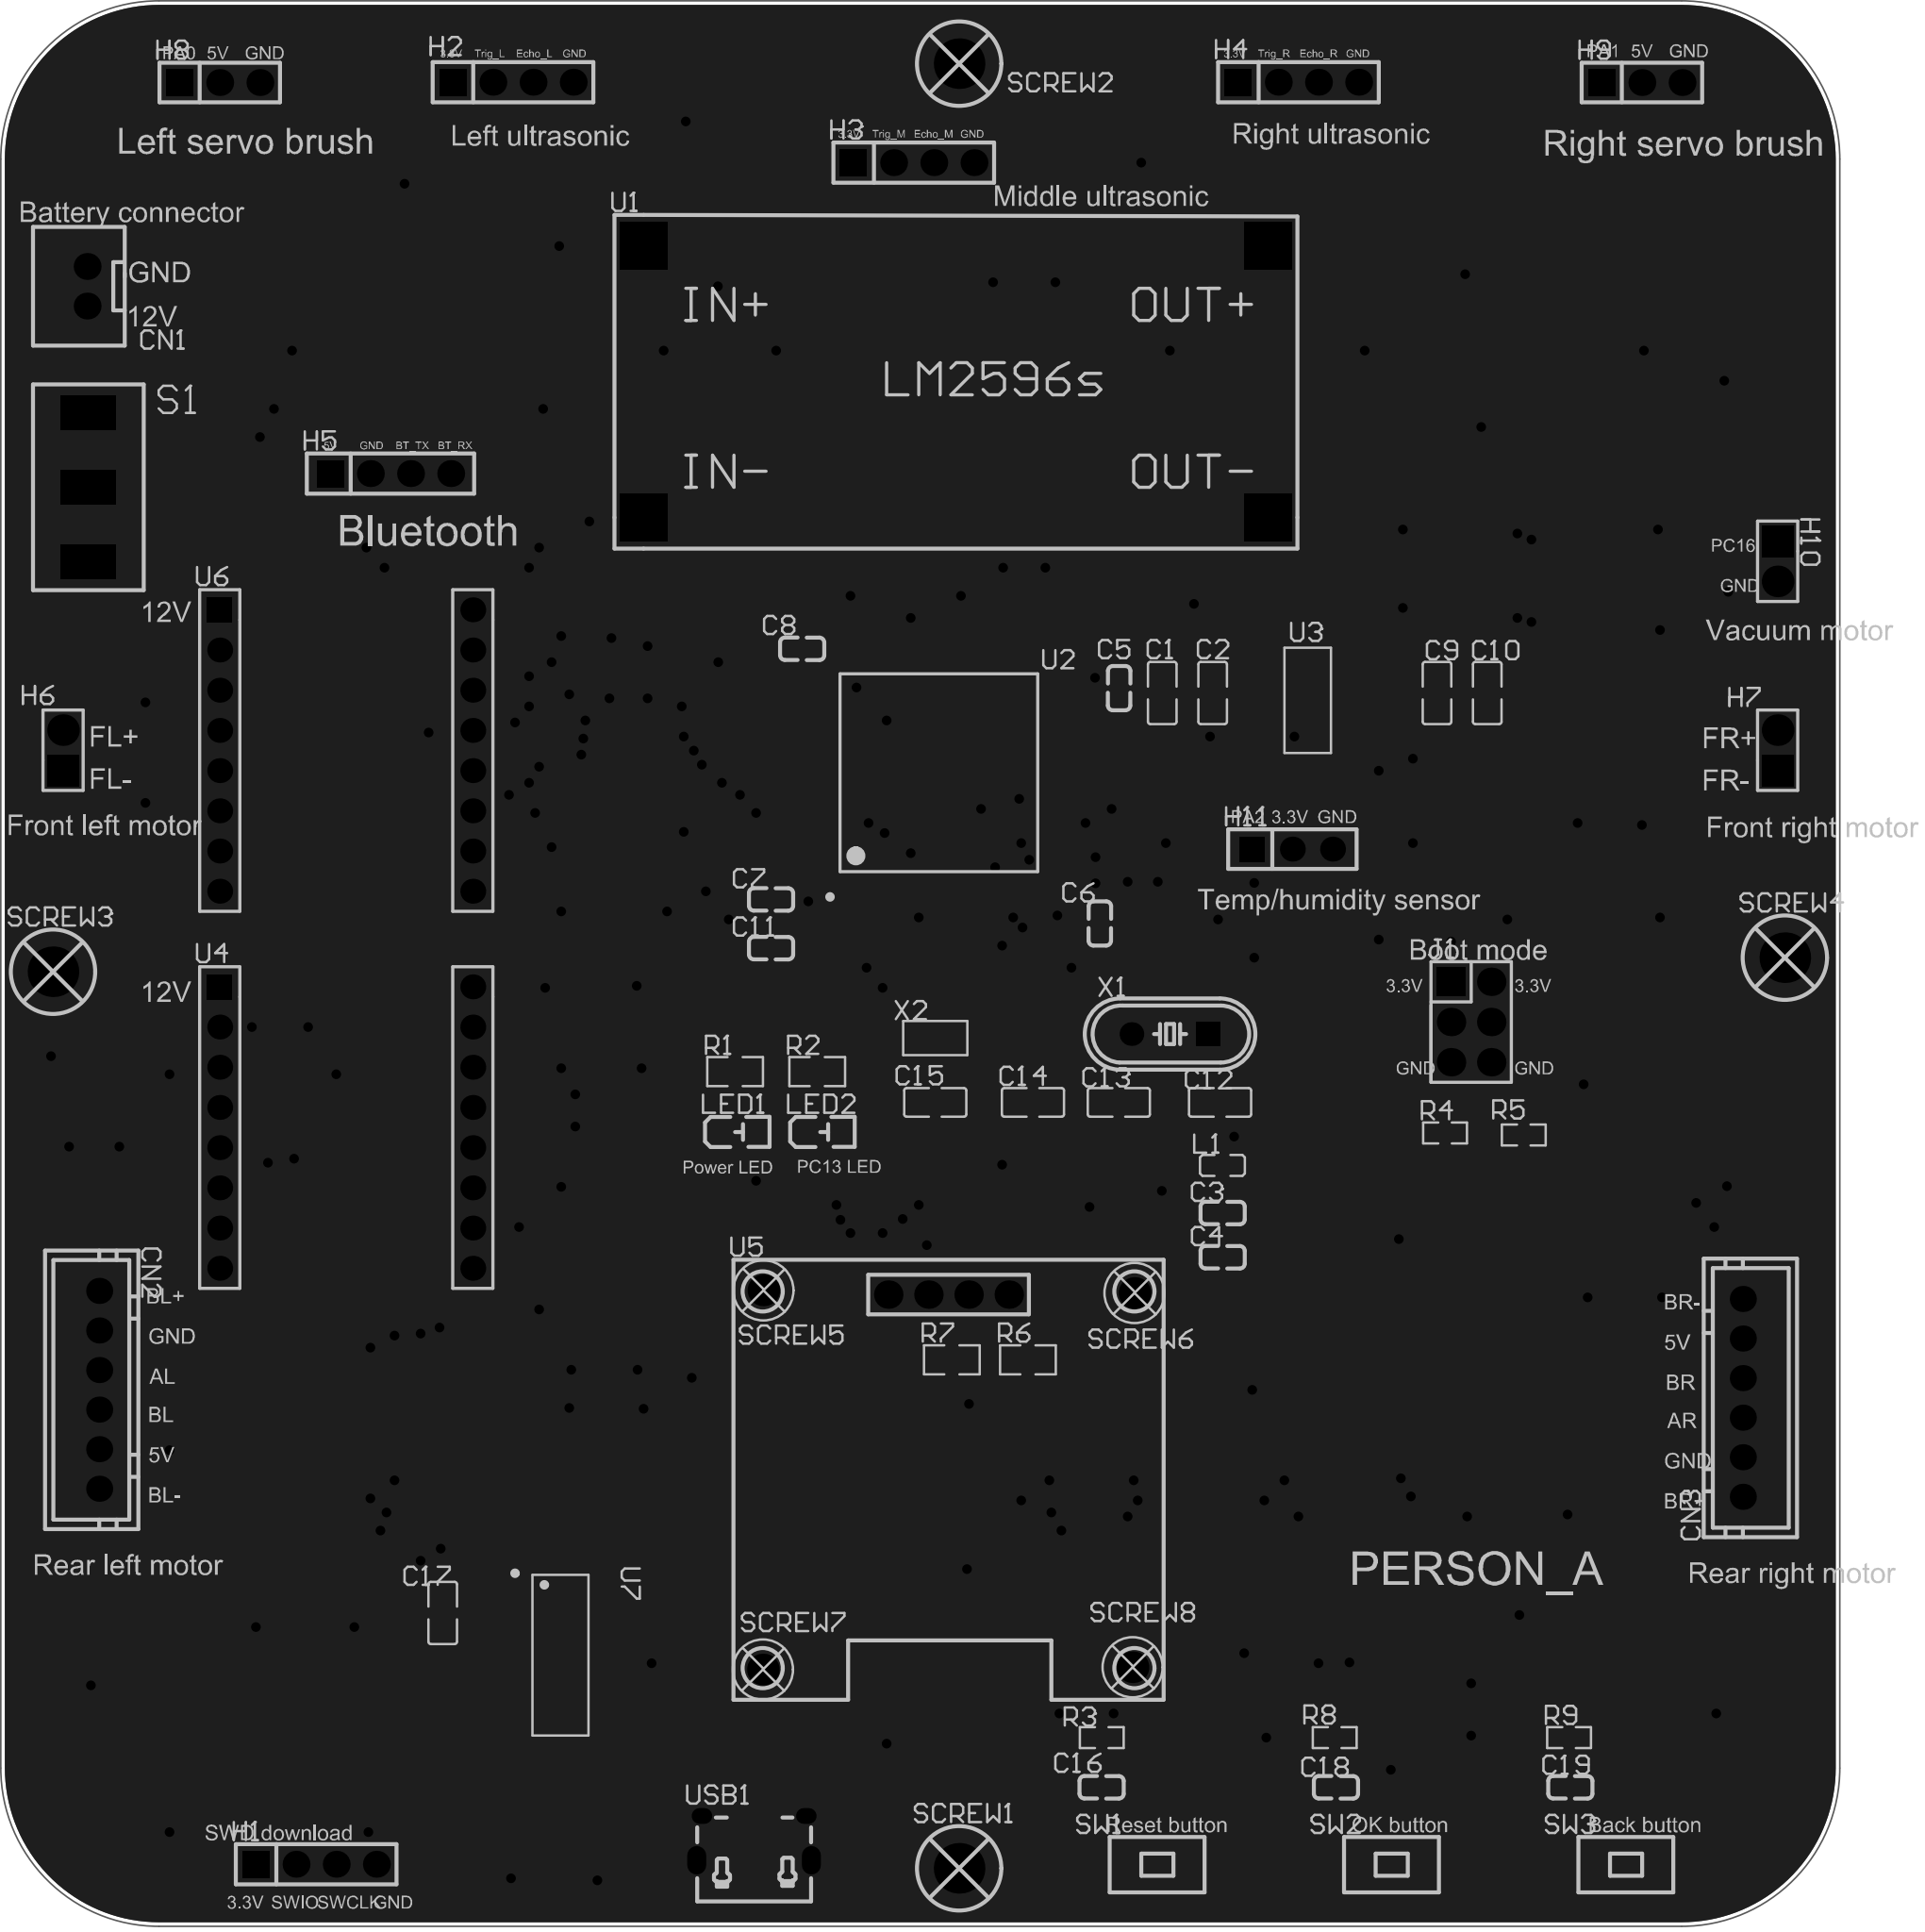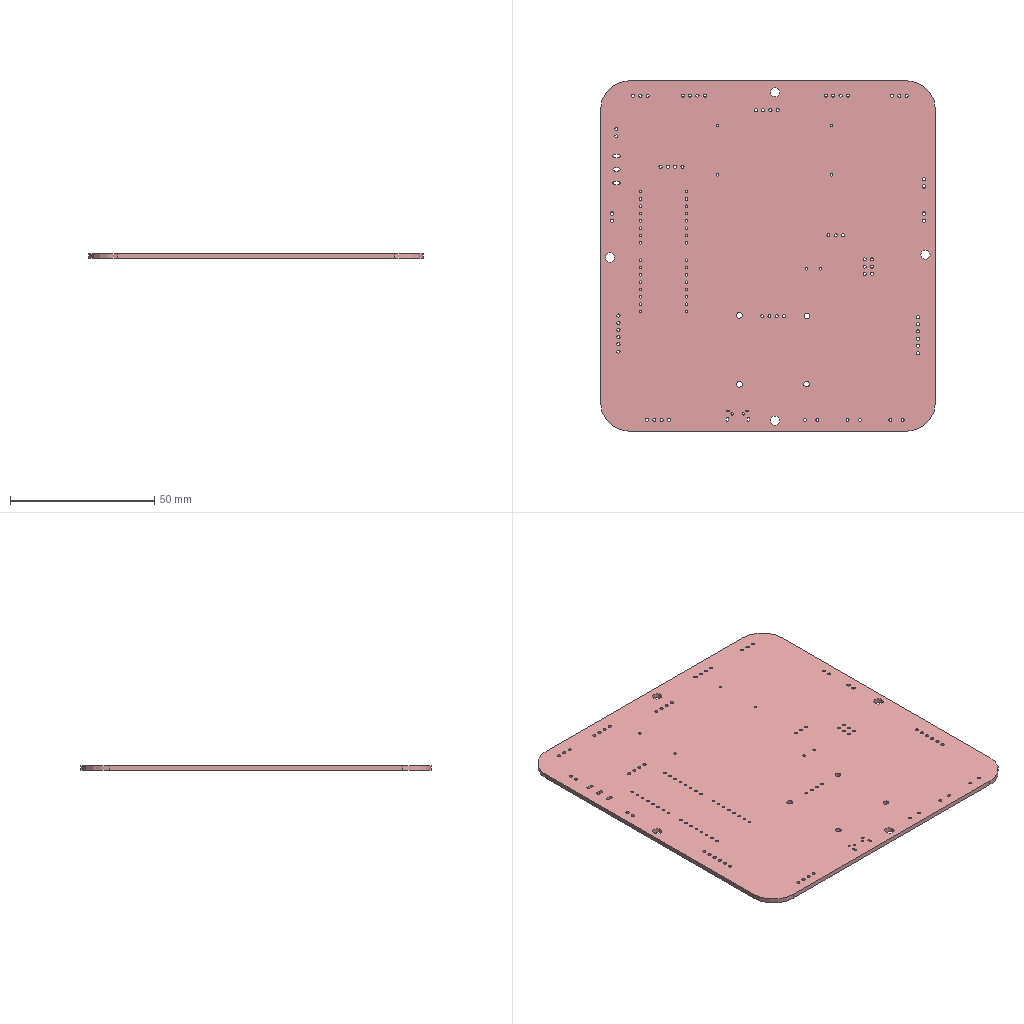Circuit board layout | Altium Designer | box 116.3 x 121.7 x 1.6 mm
Layer stack:
# Altium Designer layer stack of  (unit mm; dielectric type: 0 none, 1 core, 2 prepreg, 3 surface material)
index,name,kind,layer,copper_thickness_mm,dielectric_type,dielectric_thickness_mm,dielectric_material,dielectric_constant
0,Top Paste Mask Layer,other,,,,,,
1,Top Silkscreen Layer,other,,,,,,
2,Top Solder Mask Layer,dielectric,,,3,0.01,,3.3
3,Top Layer,copper,Top Layer,0.035,,,,
4,Dielectric1,dielectric,,,3,1.51,FR4,4.5
5,Bottom Layer,copper,Bottom Layer,0.035,,,,
6,Bottom Solder Mask Layer,dielectric,,,3,0.01,,3.3
7,Bottom Silkscreen Layer,other,,,,,,
8,Bottom Paste Mask Layer,other,,,,,,
# drill layer pairs: low layer,high layer
drill_pair,Top Layer,Bottom Layer
Part placement:
Designator,Comment,Layer,Footprint,Center-X(mm),Center-Y(mm),Rotation
C3,100nF,TopLayer,C0603,160.302,131.826,180
C4,10uF,TopLayer,C0603,160.302,129.032,180
C11,100nF,TopLayer,C0603,131.75,148.558,180
C5,100nF,TopLayer,C0603,153.762,164.975,270
C6,100nF,TopLayer,C0603,152.542,150.108,270
C7,100nF,TopLayer,C0603,131.75,151.638,180
C8,100nF,TopLayer,C0603,133.717,167.471,180
C16,1uF,TopLayer,C0603,152.649,95.543,180
CN1,XH2.54*2P_THT,TopLayer,CONN-TH_2P-P2.50-XH2.54-2P,88.519,190.373,270
CN2,Rear left motor,TopLayer,CONN-TH_XH2.54-6P,89.281,120.651,270
CN3,Rear right motor,TopLayer,CONN-TH_XH2.54-6P,193.199,120.142,90
SCREW1,,TopLayer,M3螺丝,143.65,90.421,0
H1,SWD,TopLayer,HDR-TH_4P-P2.54-V-M,102.997,90.678,0
H5,2.54-1*4P female,TopLayer,HDR-TH_4P-P2.54-V-F,107.696,178.539,0
H6,Front left motor,TopLayer,HDR-TH_2P-P2.54-V-M,86.995,161.061,90
H7,Front right motor,TopLayer,HDR-TH_2P-P2.54-V-M,195.398,161.061,90
H2,Ultrasonic left,TopLayer,HDR-TH_4P-P2.54-V-M,115.442,203.265,0
H3,Ultrasonic middle,TopLayer,HDR-TH_4P-P2.54-V-M,140.78,198.185,0
H4,Ultrasonic right,TopLayer,HDR-TH_4P-P2.54-V-M,165.101,203.265,0
H8,PZ254V-11-03P,TopLayer,HDR-TH_3P-P2.54-V-M,96.901,203.245,0
H9,PZ254V-11-03P,TopLayer,HDR-TH_3P-P2.54-V-M,186.817,203.245,0
H10,PZ254V-11-02P,TopLayer,HDR-TH_2P-P2.54-V-M,195.398,172.998,270
H11,PM254V-11-03-H85,TopLayer,HDR-TH_3P-P2.54-V-F,164.719,154.813,0
J1,2.54-2*3P male pin,TopLayer,HDR-TH_6P-P2.54-V-M-R2-C3-S2.54-1,176.022,143.891,270
L1,10uH,TopLayer,L0603,160.302,134.82,0
LED2,NCD0805R1,TopLayer,LED0805-RD_RED,135.066,136.942,0
LED1,NCD0805R1,TopLayer,LED0805-RD_RED,129.683,136.942,0
R3,10kΩ,TopLayer,R0603,152.666,98.679,0
R5,10kΩ,TopLayer,R0603,179.348,136.752,0
R4,10kΩ,TopLayer,R0603,174.371,136.879,0
R6,4.7kΩ,TopLayer,R0805,147.998,122.546,180
R7,4.7kΩ,TopLayer,R0805,143.188,122.546,180
S1,ss12d10 switch,TopLayer,SS12D10,88.594,177.673,90
SCREW2,,TopLayer,M3螺丝,143.65,204.438,0
U2,STM32F103VET6,TopLayer,LQFP-100_L14.0-W14.0-P0.50-LS16.0-BL,142.367,159.639,0
U3,AMS1117-3.3,TopLayer,SOT-223-3_L6.5-W3.4-P2.30-LS7.0-BR,165.787,164.211,0
U1,LM2596S buck module,TopLayer,LM2596S,143.446,184.34,0
U5,HS96L03W2C03,TopLayer,OLED-TH_L27.8-W27.2-P2.54_C9900033791,142.98,126.669,0
U4,TB6612 module,TopLayer,TB6612-2X8,104.901,137.222,0
U6,TB6612 module,TopLayer,TB6612-2X8,104.901,161.042,0
X1,-,TopLayer,HC-49US_L11.5-W4.5-P4.88,156.985,143.129,180
X2,32.768kHz,TopLayer,OSC-SMD_L3.2-W1.5,142.14,142.875,180
SCREW3,,TopLayer,M3螺丝,86.36,147.066,0
SCREW4,,TopLayer,M3螺丝,195.855,147.955,0
SCREW5,,TopLayer,M2螺丝,131.275,126.935,0
SCREW6,,TopLayer,M2螺丝,154.736,126.769,0
SCREW7,,TopLayer,M2螺丝,131.244,102.981,0
SCREW8,,TopLayer,M2螺丝,154.617,103.124,0
C9,10uF,TopLayer,C0805,173.863,164.675,90
C10,100nF,TopLayer,C0805,177.038,164.675,90
C1,10uF,TopLayer,C0805,156.491,164.675,90
C2,100nF,TopLayer,C0805,159.677,164.675,90
C17,100pF,TopLayer,C0805,110.998,106.553,270
C12,20pF,TopLayer,C0805,160.147,138.811,0
C13,20pF,TopLayer,C0805,153.745,138.811,0
C14,20pF,TopLayer,C0805,148.315,138.811,0
C15,20pF,TopLayer,C0805,142.14,138.811,180
SW1,1TS002C-2300-4300-CT,TopLayer,SW-SMD_L6.0-W3.5-LS8.0-EH,156.166,90.65,0
C18,1uF,TopLayer,C0603,167.466,95.543,180
C19,1uF,TopLayer,C0603,182.283,95.543,180
R8,10kΩ,TopLayer,R0603,167.395,98.679,0
R9,10kΩ,TopLayer,R0603,182.212,98.679,0
SW2,1TS002C-2300-4300-CT,TopLayer,SW-SMD_L6.0-W3.5-LS8.0-EH,170.983,90.65,0
SW3,1TS002C-2300-4300-CT,TopLayer,SW-SMD_L6.0-W3.5-LS8.0-EH,185.801,90.65,0
U7,CH340C,TopLayer,SOP-16_L10.0-W3.9-P1.27-LS6.0-BL,118.443,103.886,270
USB1,USB Android female socket,TopLayer,MICRO-USB-SMD_MICRO-USB-A8,130.683,92.329,0
R1,680Ω,TopLayer,R0805,129.484,140.757,0
R2,680Ω,TopLayer,R0805,134.676,140.757,0
Pad and via stacks:
# Altium Designer via and pad stacks of  (unit mm). Each distinct definition once, with the count of objects using it.
# via: kind,start_layer,end_layer,hole_mm,diameter_mm,mode(0 simple;1 top-mid-bottom;2 full stack),diameter_per_layer,count,example_net
# pad: kind,layer,hole_mm,hole_type(0 round;1 square;2 slot),plating,top_size,top_shape(1 round;2 rect;3 octagon;9 rounded rect),mid_size,bottom_size,mode,footprint,size_per_layer,count,example
pad,Top Layer,0,0,plated,0.8x0.9,2,0.8x0.9,0.8x0.9,0,C0603,,20,C3.2
pad,Top Layer,0,0,plated,0.8x0.864,2,0.8x0.864,0.8x0.864,0,L0603,,2,L1.1
pad,Top Layer,0,0,plated,1x1.25,2,1x1.25,1x1.25,0,LED0805-RD_RED,,4,LED2.2
pad,Top Layer,0,0,plated,0.8065x0.864,2,0.8065x0.864,0.8065x0.864,0,R0603,,10,R3.2
pad,Top Layer,0,0,plated,1.133x1.377,2,1.133x1.377,1.133x1.377,0,R0805,,8,R6.2
pad,Top Layer,0,0,plated,1.6x0.3,1,1.6x0.3,1.6x0.3,0,LQFP-100_L14.0-W14.0-P0.50-LS16.0-BL,,50,U2.100
pad,Top Layer,0,0,plated,0.3x1.6,1,0.3x1.6,0.3x1.6,0,LQFP-100_L14.0-W14.0-P0.50-LS16.0-BL,,50,U2.75
pad,Top Layer,0,0,plated,2.5x1.1,2,2.5x1.1,2.5x1.1,0,SOT-223-3_L6.5-W3.4-P2.30-LS7.0-BR,,3,U3.1
pad,Top Layer,0,0,plated,2.34x3.6,2,2.34x3.6,2.34x3.6,0,SOT-223-3_L6.5-W3.4-P2.30-LS7.0-BR,,1,U3.4
pad,Top Layer,0,0,plated,1.05x1.7,2,1.05x1.7,1.05x1.7,0,OSC-SMD_L3.2-W1.5,,2,X2.1
pad,Top Layer,0,0,plated,1.41x1.35,2,1.41x1.35,1.41x1.35,0,C0805,,18,C9.2
pad,Top Layer,0,0,plated,1.9x1.7,2,1.9x1.7,1.9x1.7,0,SW-SMD_L6.0-W3.5-LS8.0-EH,,6,SW1.1
pad,Top Layer,0,0,plated,0.56x1.745,1,0.56x1.745,0.56x1.745,0,SOP-16_L10.0-W3.9-P1.27-LS6.0-BL,,16,U7.1
pad,Top Layer,0,0,plated,1.5x0.45,2,1.5x0.45,1.5x0.45,0,MICRO-USB-SMD_MICRO-USB-A8,,5,USB1.5
pad,Multi-Layer,1.05,0,plated,1.7x1.7,1,1.7x1.7,1.7x1.7,0,CONN-TH_2P-P2.50-XH2.54-2P,,2,CN1.2
pad,Multi-Layer,1.1,0,plated,1.65x1.65,1,1.65x1.65,1.65x1.65,0,CONN-TH_XH2.54-6P,,12,CN2.1
pad,Multi-Layer,3.2,0,plated,3.2x3.2,1,3.2x3.2,3.2x3.2,0,M3\u00C2\u00DD\u00CB\u00BF,,4,SCREW1.1
pad,Multi-Layer,1.1,0,plated,1.7x1.7,2,1.7x1.7,1.7x1.7,0,HDR-TH_4P-P2.54-V-M,,4,H1.1
pad,Multi-Layer,1.1,0,plated,1.7x1.7,1,1.7x1.7,1.7x1.7,0,HDR-TH_4P-P2.54-V-M,,12,H1.2
pad,Multi-Layer,1.1,0,plated,1.7x1.7,2,1.7x1.7,1.7x1.7,0,HDR-TH_4P-P2.54-V-F,,1,H5.1
pad,Multi-Layer,1.1,0,plated,1.7x1.7,1,1.7x1.7,1.7x1.7,0,HDR-TH_4P-P2.54-V-F,,3,H5.2
pad,Multi-Layer,1.2,0,plated,2x2,2,2x2,2x2,0,HDR-TH_2P-P2.54-V-M,,3,H6.1
pad,Multi-Layer,1.2,0,plated,2x2,1,2x2,2x2,0,HDR-TH_2P-P2.54-V-M,,3,H6.2
pad,Multi-Layer,1.1,0,plated,1.7x1.7,2,1.7x1.7,1.7x1.7,0,HDR-TH_3P-P2.54-V-M,,2,H8.1
pad,Multi-Layer,1.1,0,plated,1.7x1.7,1,1.7x1.7,1.7x1.7,0,HDR-TH_3P-P2.54-V-M,,4,H8.2
pad,Multi-Layer,1.02,0,plated,1.575x1.575,1,1.575x1.575,1.575x1.575,0,HDR-TH_3P-P2.54-V-F,,2,H11.3
pad,Multi-Layer,1.02,0,plated,1.575x1.575,2,1.575x1.575,1.575x1.575,0,HDR-TH_3P-P2.54-V-F,,1,H11.1
pad,Multi-Layer,1.05,0,plated,1.8x1.8,1,1.8x1.8,1.8x1.8,0,HDR-TH_6P-P2.54-V-M-R2-C3-S2.54-1,,5,J1.6
pad,Multi-Layer,1.05,0,plated,1.8x1.8,2,1.8x1.8,1.8x1.8,0,HDR-TH_6P-P2.54-V-M-R2-C3-S2.54-1,,1,J1.1
pad,Multi-Layer,1.199,2,plated,2.2x3.5,2,2.2x3.5,2.2x3.5,0,SS12D10,,3,S1.3
pad,Multi-Layer,0.9144,0,plated,3x3,2,3x3,3x3,0,LM2596S,,4,U1.4
pad,Multi-Layer,1.05,0,plated,1.8x1.8,1,1.8x1.8,1.8x1.8,0,OLED-TH_L27.8-W27.2-P2.54_C9900033791,,4,U5.1
pad,Multi-Layer,0.889,0,plated,1.575x1.575,1,1.575x1.575,1.575x1.575,0,TB6612-2X8,,30,U4.8
pad,Multi-Layer,0.889,0,plated,1.575x1.575,2,1.575x1.575,1.575x1.575,0,TB6612-2X8,,2,U4.1
pad,Multi-Layer,0.9,0,plated,1.5x1.5,2,1.5x1.5,1.5x1.5,0,HC-49US_L11.5-W4.5-P4.88,,1,X1.1
pad,Multi-Layer,0.9,0,plated,1.5x1.5,1,1.5x1.5,1.5x1.5,0,HC-49US_L11.5-W4.5-P4.88,,1,X1.2
pad,Multi-Layer,2,0,plated,2x2,1,2x2,2x2,0,M2\u00C2\u00DD\u00CB\u00BF,,4,SCREW5.1
pad,Multi-Layer,0.6,2,plated,1.3x1,1,1.3x1,1.3x1,0,MICRO-USB-SMD_MICRO-USB-A8,,2,USB1.6
pad,Multi-Layer,0.8,2,plated,1.8x1.2,1,1.8x1.2,1.8x1.2,0,MICRO-USB-SMD_MICRO-USB-A8,,2,USB1.8
via,Top Layer,Bottom Layer,0.3048,0.61,0,,204,PC6
Copper pours:
name,layer,net,type(0 solid;1 hatched;2 none)
Top Layer-GND,Top Layer,GND,0
Bottom Layer-GND,Bottom Layer,GND,0